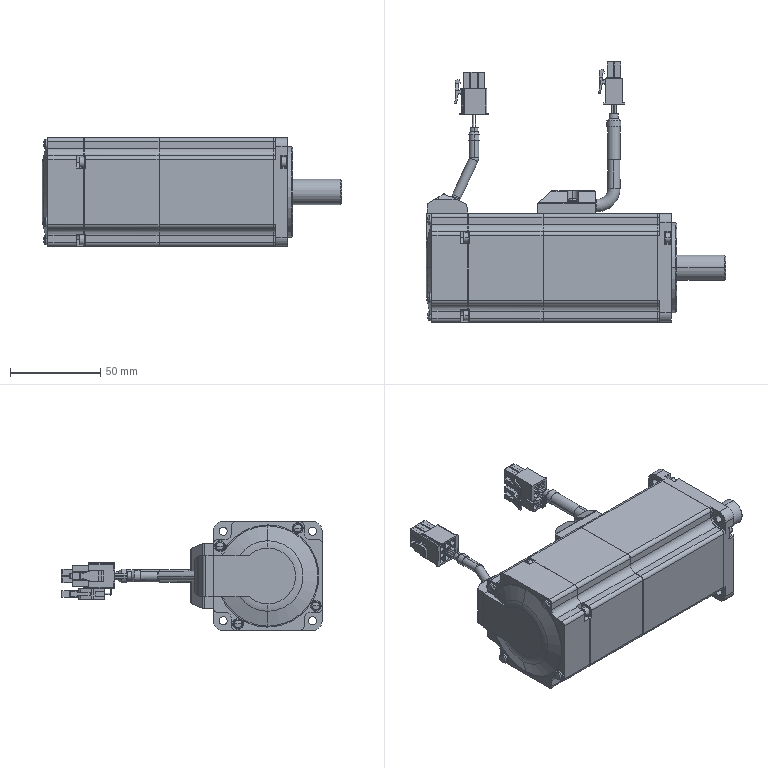Part | STEP file | 001-003-MSMF042L1D2 | 8 solids | 1063 faces | box 165.5 x 143.937 x 60 mm | volume 465510 mm3 | plane 632 | cylinder 320 | cone 59 | torus 36 | sphere 12 | other 4 | commonest cylinder face diameters 1 x47 4 x33 2.6 x30 6 x29 3.92 x20 5.5 x16